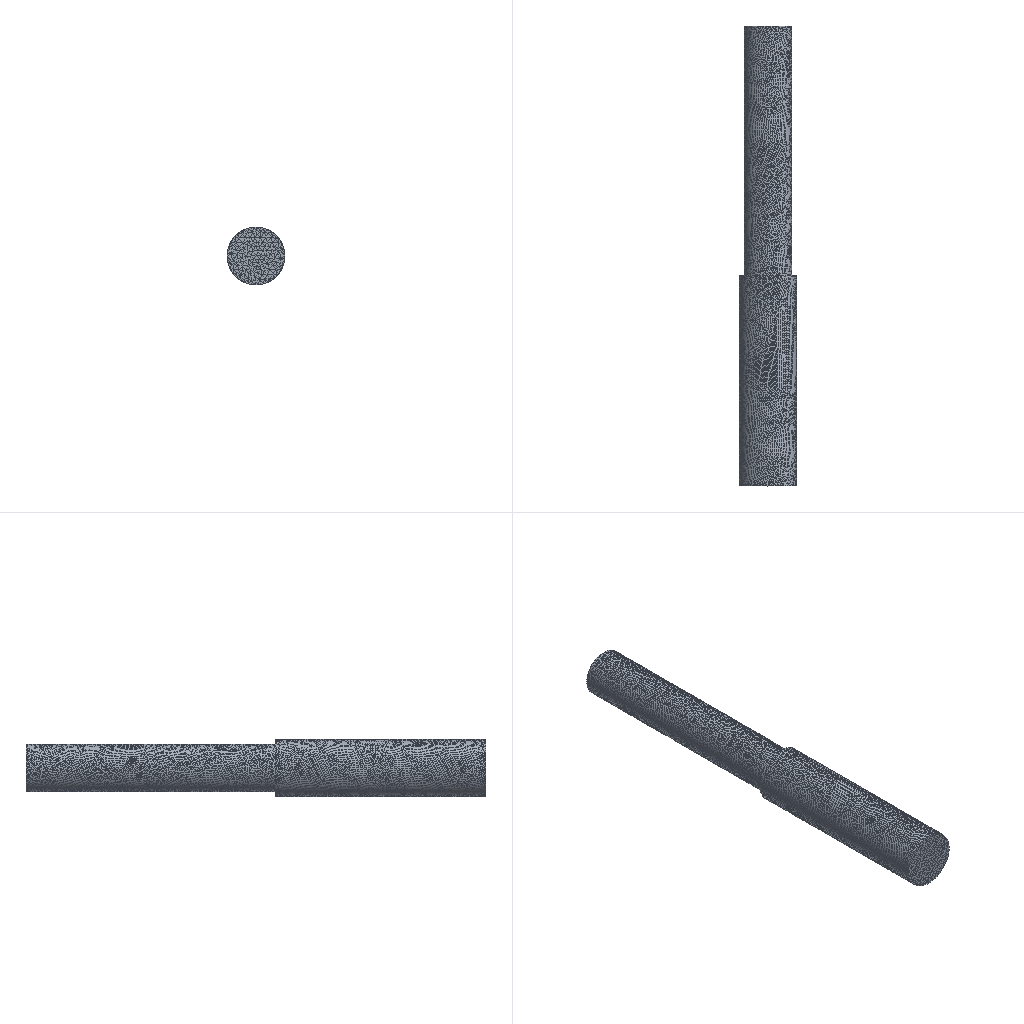Simulation study | ansys workbench
Ansys APDL input file, long lists of numbers shortened:
/batch
/config,noeldb,1     ! force off writing results to database
*get,_wallstrt,active,,time,wall
! ANSYS input file written by Workbench version 2022 R1
! File used for geometry attach: F:\ansys（分析文件汇总)\ansys有限元题目分析\1_files\dp0\SYS-2\DM\SYS-2.scdoc
/title,1--____ (C5)
! ****** Begin Custom Load Command Snippet ******
/COM, ACT Extensions:
/COM,     LSDYNA, 2021.1
/COM,
! ****** End   Custom Load Command Snippet ******
*DIM,_wb_ProjectScratch_dir,string,248
_wb_ProjectScratch_dir(1) = 'F:\ansys（分析文件汇总)\ansys有限元题目分析\_ProjectScratch\ScrBC79\'
*DIM,_wb_SolverFiles_dir,string,248
_wb_SolverFiles_dir(1) = 'F:\ansys（分析文件汇总)\ansys有限元题目分析\1_files\dp0\SYS-2\MECH\'
*DIM,_wb_userfiles_dir,string,248
_wb_userfiles_dir(1) = 'F:\ansys（分析文件汇总)\ansys有限元题目分析\1_files\user_files\'
/com,--- Data in consistent NMM units. See Solving Units in the help system for more information.
/units,MPA
/nopr
/wb,file,start              !  signify a WB generated input file
/prep7
! Turn off shape checking because checks already performed inside WB mesher.
! See help system for more information.
SHPP,OFF,,NOWARN
/nolist
etcon,set             ! allow ANSYS to choose best KEYOP's for 180x elements, resets any applicable keyopt to MAPDL defaults
/com,*********** Nodes for the whole assembly ***********
nblock,3,,432
(1i9,3e20.9e3)
        1     4.600000000E+01     5.000000000E+01    -2.500000000E+01
! (392 more lines like these left out)
-1
/wb,elem,start            !  set before creation of elements
/com,*********** Elements for Body 1 "SYS-2\__" ***********
et,1,186
keyo,1,2,1          ! set full integration on SOLID186
eblock,19,solid,,40
(19i9)
        1        1        1        1        0        0        0        0       20        0        1       19      125      124      122       20       40       41       42
! (79 more lines like these left out)
-1
/wb,elem,end               !  done creating elements
/com,*********** Send User Defined Coordinate System(s) ***********
csys,0
toffst,273.15,  ! Temperature offset from absolute zero
/com,*********** Set Reference Temperature ***********
tref,22.
/wb,mat,start              !  starting to send materials
/com,*********** Send Materials ***********
Temperature = 'TEMP' ! Temperature
MP,DENS,1,7.85e-09,	! tonne mm^-3
MP,ALPX,1,1.2e-05,	! C^-1
MP,C,1,434000000,	! mm^2 s^-2 C^-1
MP,KXX,1,60.5,	! tonne mm s^-3 C^-1
MP,RSVX,1,0.00017,	! ohm mm
MP,EX,1,200000,	! tonne s^-2 mm^-1
MP,NUXY,1,0.3,
MP,MURX,1,10000,
/wb,mat,end                !  done sending materials
!************************* Model Summary ********************
!SYS-2\__,	结构钢,	matid,	1
!************************* End Model Summary ********************
! get the diagonal of the bounding box. Needed later for other things
*get,_xmin,node,,mnloc,x
*get,_ymin,node,,mnloc,y
*get,_zmin,node,,mnloc,z
*get,_xmax,node,,mxloc,x
*get,_ymax,node,,mxloc,y
*get,_zmax,node,,mxloc,z
_ASMDIAG=(_xmax-_xmin)*(_xmax-_xmin)+(_ymax-_ymin)*(_ymax-_ymin)+(_zmax-_zmin)*(_zmax-_zmin)
_ASMDIAG=SQRT(_ASMDIAG)
/wb,contact,start          !  starting to send contact
/wb,contact,end            !  done creating contacts
/golist
/wb,load,start             !  starting to send loads
/com,*********** Fixed Supports ***********
CMBLOCK,_FIXEDSU,NODE,       13
(8i10)
        40        41        62       103       124       125       265       266
       267       269       310       371       393
cmsel,s,_FIXEDSU
d,all,all
nsel,all
/com,*********** Define Force Using Surface Effect Elements ***********
local,12,0,0.,0.,0.,0.,0.,0.
csys,0
et,2,156
keyop,2,5,1         !  No orientation node
eblock,10,,,1
(15i9)
      165        2        2        2       12      123       61      308
-1
esel,s,type,,2
keyop,2,2,1                ! Apply load in local coordinate system
keyop,2,7,1                ! Use original area so load is constant in large deformation
esel,all
/gst,on,on
fini
*get,_numnode,node,0,count
*get,_numelem,elem,0,count
*get, _MAXELEMNUM, elem, 0, NUM, MAX
*get, _MAXNODENUM, node, 0, NUM, MAX
*get, _MAXELEMTYPE, etyp, 0, NUM, MAX
*get, _MAXREALCONST, real, 0, NUM, MAX
/go
/wb,load,end               !  done creating loads
/com,--- Number of total nodes = %_numnode%
/com,--- Number of contact elements = 1
/com,--- Number of spring elements = 0
/com,--- Number of bearing elements = 0
/com,--- Number of solid elements = 40
/com,--- Number of condensed parts = 0
/com,--- Number of total elements = %_numelem%
*get,_wallbsol,active,,time,wall
/com,****************************************************************************
/com,*************************    SOLUTION       ********************************
/com,****************************************************************************
/solu
antype,0                   ! static analysis
_thickRatio=  0     ! Ratio of thick parts in the model
eqsl,sparse,,,,,1
cntr,print,1               ! print out contact info and also make no initial contact an error
dmpoption,emat,no             ! Don't combine emat file for DANSYS
dmpoption,esav,no             ! Don't combine esav file for DANSYS
nldiag,cont,iter           ! print out contact info each equilibrium iteration
rescontrol,,none                 ! Do not keep any restart files
/com,****************************************************
/com,******************* SOLVE FOR LS 1 OF 1 ****************
esel,s,type,,2
nsle
sfe,all,1,pres,1,200.
sfe,all,2,pres,1,0.
sfe,all,3,pres,1,0.
nsel,all
esel,all
/nopr
/gopr
nsub,1,1,1
time,1.
outres,erase
outres,all,none
outres,nsol,all,
outres,rsol,all
outres,eangl,all
outres,etmp,all
outres,veng,all
outres,strs,all,
outres,epel,all,
outres,eppl,all,
outres,cont,all,
! *********** WB SOLVE COMMAND ***********
! check interactive state
*get,ANSINTER_,active,,int
*if,ANSINTER_,ne,0,then
/eof
*endif
solve
/com *************** Write FE CONNECTORS *********
CEWRITE,file,ce,,INTE
/com,****************************************************
/com,*************** FINISHED SOLVE FOR LS 1 *************
*get,_wallasol,active,,time,wall
/nopr
*get,_numnode,node,0,count
*get,_numelem,elem,0,count
*get, _MAXELEMNUM, elem, 0, NUM, MAX
*get, _MAXNODENUM, node, 0, NUM, MAX,,,INTERNAL
*get, _MAXELEMTYPE, etyp, 0, NUM, MAX
*get, _MAXREALCONST, real, 0, NUM, MAX
/gopr
/post1
xmlo,ENCODING,ISO-8859-1
xmlo,parm
/xml,parm,xml
fini
/gopr
*get,_walldone,active,,time,wall
_preptime=(_wallbsol-_wallstrt)*3600
_solvtime=(_wallasol-_wallbsol)*3600
_posttime=(_walldone-_wallasol)*3600
_totaltim=(_walldone-_wallstrt)*3600
*get,_dlbratio,active,0,solu,dlbr
*get,_combtime,active,0,solu,comb
*get,_ssmode,active,0,solu,ssmm
*get,_ndofs,active,0,solu,ndof
*get,_sol_end_time,active,0,set,time
*if,_sol_end_time,eq,1.,then
/fclean				!clean distributed files
*endif
/com,--- Total number of nodes = %_numnode%
/com,--- Total number of elements = %_numelem%
/com,--- Element load balance ratio = %_dlbratio%
/com,--- Time to combine distributed files = %_combtime%
/com,--- Sparse memory mode = %_ssmode%
/com,--- Number of DOF = %_ndofs%
/wb,file,end               ! done with WB generated input